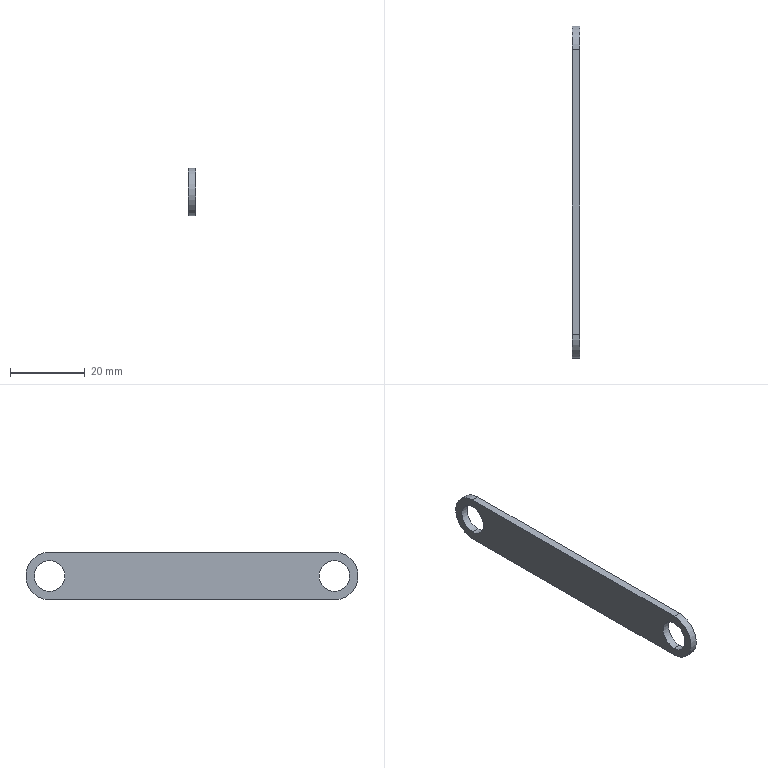Part | SolidWorks | features Extrusion 1 | 1 solid | 10 faces | box 2 x 88.9 x 12.7 mm | volume 1978 mm3 | cylinder 6 | plane 4 | commonest cylinder face diameters 8.2 x4 12.7 x2
STEP:
#1=CARTESIAN_POINT('',(2.,-38.1,4.1));
#2=VERTEX_POINT('',#1);
#3=CARTESIAN_POINT('',(2.,-38.1,-4.1));
#4=VERTEX_POINT('',#3);
#5=CARTESIAN_POINT('',(2.,-38.1,0.));
#6=DIRECTION('',(1.,0.,0.));
#7=DIRECTION('',(0.,0.,-1.));
#8=AXIS2_PLACEMENT_3D('',#5,#6,#7);
#9=CIRCLE('',#8,4.1);
#10=EDGE_CURVE('',#2,#4,#9,.T.);
#11=ORIENTED_EDGE('',*,*,#10,.T.);
#12=CARTESIAN_POINT('',(0.,-38.1,-4.1));
#13=VERTEX_POINT('',#12);
#14=CARTESIAN_POINT('',(2.,-38.1,-4.1));
#15=DIRECTION('',(-1.,0.,0.));
#16=VECTOR('',#15,1000.);
#17=LINE('',#14,#16);
#18=EDGE_CURVE('',#4,#13,#17,.T.);
#19=ORIENTED_EDGE('',*,*,#18,.T.);
#20=CARTESIAN_POINT('',(0.,-38.1,4.1));
#21=VERTEX_POINT('',#20);
#22=CARTESIAN_POINT('',(0.,-38.1,0.));
#23=DIRECTION('',(1.,0.,0.));
#24=DIRECTION('',(0.,0.,-1.));
#25=AXIS2_PLACEMENT_3D('',#22,#23,#24);
#26=CIRCLE('',#25,4.1);
#27=EDGE_CURVE('',#21,#13,#26,.T.);
#28=ORIENTED_EDGE('',*,*,#27,.F.);
#29=CARTESIAN_POINT('',(2.,-38.1,4.1));
#30=DIRECTION('',(-1.,0.,0.));
#31=VECTOR('',#30,1000.);
#32=LINE('',#29,#31);
#33=EDGE_CURVE('',#2,#21,#32,.T.);
#34=ORIENTED_EDGE('',*,*,#33,.F.);
#35=EDGE_LOOP('',(#11,#19,#28,#34));
#36=FACE_OUTER_BOUND('',#35,.T.);
#37=CARTESIAN_POINT('',(2.,-38.1,0.));
#38=DIRECTION('',(-1.,0.,0.));
#39=DIRECTION('',(0.,0.,1.));
#40=AXIS2_PLACEMENT_3D('',#37,#38,#39);
#41=CYLINDRICAL_SURFACE('',#40,4.1);
#42=ADVANCED_FACE('',(#36),#41,.F.);
#43=CARTESIAN_POINT('',(2.,38.1,4.1));
#44=VERTEX_POINT('',#43);
#45=CARTESIAN_POINT('',(2.,38.1,-4.1));
#46=VERTEX_POINT('',#45);
#47=CARTESIAN_POINT('',(2.,38.1,0.));
#48=DIRECTION('',(1.,0.,0.));
#49=DIRECTION('',(0.,0.,-1.));
#50=AXIS2_PLACEMENT_3D('',#47,#48,#49);
#51=CIRCLE('',#50,4.1);
#52=EDGE_CURVE('',#44,#46,#51,.T.);
#53=ORIENTED_EDGE('',*,*,#52,.T.);
#54=CARTESIAN_POINT('',(0.,38.1,-4.1));
#55=VERTEX_POINT('',#54);
#56=CARTESIAN_POINT('',(2.,38.1,-4.1));
#57=DIRECTION('',(-1.,0.,0.));
#58=VECTOR('',#57,1000.);
#59=LINE('',#56,#58);
#60=EDGE_CURVE('',#46,#55,#59,.T.);
#61=ORIENTED_EDGE('',*,*,#60,.T.);
#62=CARTESIAN_POINT('',(0.,38.1,4.1));
#63=VERTEX_POINT('',#62);
#64=CARTESIAN_POINT('',(0.,38.1,0.));
#65=DIRECTION('',(1.,0.,0.));
#66=DIRECTION('',(0.,0.,-1.));
#67=AXIS2_PLACEMENT_3D('',#64,#65,#66);
#68=CIRCLE('',#67,4.1);
#69=EDGE_CURVE('',#63,#55,#68,.T.);
#70=ORIENTED_EDGE('',*,*,#69,.F.);
#71=CARTESIAN_POINT('',(2.,38.1,4.1));
#72=DIRECTION('',(-1.,0.,0.));
#73=VECTOR('',#72,1000.);
#74=LINE('',#71,#73);
#75=EDGE_CURVE('',#44,#63,#74,.T.);
#76=ORIENTED_EDGE('',*,*,#75,.F.);
#77=EDGE_LOOP('',(#53,#61,#70,#76));
#78=FACE_OUTER_BOUND('',#77,.T.);
#79=CARTESIAN_POINT('',(2.,38.1,0.));
#80=DIRECTION('',(-1.,0.,0.));
#81=DIRECTION('',(0.,0.,1.));
#82=AXIS2_PLACEMENT_3D('',#79,#80,#81);
#83=CYLINDRICAL_SURFACE('',#82,4.1);
#84=ADVANCED_FACE('',(#78),#83,.F.);
#85=ORIENTED_EDGE('',*,*,#52,.F.);
#86=CARTESIAN_POINT('',(2.,38.1,0.));
#87=DIRECTION('',(1.,0.,0.));
#88=DIRECTION('',(0.,0.,-1.));
#89=AXIS2_PLACEMENT_3D('',#86,#87,#88);
#90=CIRCLE('',#89,4.1);
#91=EDGE_CURVE('',#46,#44,#90,.T.);
#92=ORIENTED_EDGE('',*,*,#91,.F.);
#93=EDGE_LOOP('',(#85,#92));
#94=FACE_BOUND('',#93,.T.);
#95=CARTESIAN_POINT('',(2.,-38.1,6.35));
#96=VERTEX_POINT('',#95);
#97=CARTESIAN_POINT('',(2.,-38.1,-6.35));
#98=VERTEX_POINT('',#97);
#99=CARTESIAN_POINT('',(2.,-38.1,0.));
#100=DIRECTION('',(1.,0.,0.));
#101=DIRECTION('',(0.,0.,-1.));
#102=AXIS2_PLACEMENT_3D('',#99,#100,#101);
#103=CIRCLE('',#102,6.35);
#104=EDGE_CURVE('',#96,#98,#103,.T.);
#105=ORIENTED_EDGE('',*,*,#104,.T.);
#106=CARTESIAN_POINT('',(2.,38.1,-6.35));
#107=VERTEX_POINT('',#106);
#108=CARTESIAN_POINT('',(2.,-38.1,-6.35));
#109=DIRECTION('',(0.,1.,0.));
#110=VECTOR('',#109,1000.);
#111=LINE('',#108,#110);
#112=EDGE_CURVE('',#98,#107,#111,.T.);
#113=ORIENTED_EDGE('',*,*,#112,.T.);
#114=CARTESIAN_POINT('',(2.,38.1,6.35));
#115=VERTEX_POINT('',#114);
#116=CARTESIAN_POINT('',(2.,38.1,0.));
#117=DIRECTION('',(1.,0.,0.));
#118=DIRECTION('',(0.,0.,-1.));
#119=AXIS2_PLACEMENT_3D('',#116,#117,#118);
#120=CIRCLE('',#119,6.35);
#121=EDGE_CURVE('',#107,#115,#120,.T.);
#122=ORIENTED_EDGE('',*,*,#121,.T.);
#123=CARTESIAN_POINT('',(2.,-38.1,6.35));
#124=DIRECTION('',(0.,-1.,0.));
#125=VECTOR('',#124,1000.);
#126=LINE('',#123,#125);
#127=EDGE_CURVE('',#115,#96,#126,.T.);
#128=ORIENTED_EDGE('',*,*,#127,.T.);
#129=EDGE_LOOP('',(#105,#113,#122,#128));
#130=FACE_OUTER_BOUND('',#129,.T.);
#131=ORIENTED_EDGE('',*,*,#10,.F.);
#132=CARTESIAN_POINT('',(2.,-38.1,0.));
#133=DIRECTION('',(1.,0.,0.));
#134=DIRECTION('',(0.,0.,-1.));
#135=AXIS2_PLACEMENT_3D('',#132,#133,#134);
#136=CIRCLE('',#135,4.1);
#137=EDGE_CURVE('',#4,#2,#136,.T.);
#138=ORIENTED_EDGE('',*,*,#137,.F.);
#139=EDGE_LOOP('',(#131,#138));
#140=FACE_BOUND('',#139,.T.);
#141=CARTESIAN_POINT('',(2.,-38.1,0.));
#142=DIRECTION('',(1.,0.,0.));
#143=DIRECTION('',(0.,0.,-1.));
#144=AXIS2_PLACEMENT_3D('',#141,#142,#143);
#145=PLANE('',#144);
#146=ADVANCED_FACE('',(#94,#130,#140),#145,.T.);
#147=CARTESIAN_POINT('',(0.,-38.1,6.35));
#148=VERTEX_POINT('',#147);
#149=CARTESIAN_POINT('',(0.,-38.1,-6.35));
#150=VERTEX_POINT('',#149);
#151=CARTESIAN_POINT('',(0.,-38.1,0.));
#152=DIRECTION('',(1.,0.,0.));
#153=DIRECTION('',(0.,0.,-1.));
#154=AXIS2_PLACEMENT_3D('',#151,#152,#153);
#155=CIRCLE('',#154,6.35);
#156=EDGE_CURVE('',#148,#150,#155,.T.);
#157=ORIENTED_EDGE('',*,*,#156,.F.);
#158=CARTESIAN_POINT('',(0.,38.1,6.35));
#159=VERTEX_POINT('',#158);
#160=CARTESIAN_POINT('',(0.,-38.1,6.35));
#161=DIRECTION('',(0.,-1.,0.));
#162=VECTOR('',#161,1000.);
#163=LINE('',#160,#162);
#164=EDGE_CURVE('',#159,#148,#163,.T.);
#165=ORIENTED_EDGE('',*,*,#164,.F.);
#166=CARTESIAN_POINT('',(0.,38.1,-6.35));
#167=VERTEX_POINT('',#166);
#168=CARTESIAN_POINT('',(0.,38.1,0.));
#169=DIRECTION('',(1.,0.,0.));
#170=DIRECTION('',(0.,0.,-1.));
#171=AXIS2_PLACEMENT_3D('',#168,#169,#170);
#172=CIRCLE('',#171,6.35);
#173=EDGE_CURVE('',#167,#159,#172,.T.);
#174=ORIENTED_EDGE('',*,*,#173,.F.);
#175=CARTESIAN_POINT('',(0.,-38.1,-6.35));
#176=DIRECTION('',(0.,1.,0.));
#177=VECTOR('',#176,1000.);
#178=LINE('',#175,#177);
#179=EDGE_CURVE('',#150,#167,#178,.T.);
#180=ORIENTED_EDGE('',*,*,#179,.F.);
#181=EDGE_LOOP('',(#157,#165,#174,#180));
#182=FACE_OUTER_BOUND('',#181,.T.);
#183=ORIENTED_EDGE('',*,*,#69,.T.);
#184=CARTESIAN_POINT('',(0.,38.1,0.));
#185=DIRECTION('',(1.,0.,0.));
#186=DIRECTION('',(0.,0.,-1.));
#187=AXIS2_PLACEMENT_3D('',#184,#185,#186);
#188=CIRCLE('',#187,4.1);
#189=EDGE_CURVE('',#55,#63,#188,.T.);
#190=ORIENTED_EDGE('',*,*,#189,.T.);
#191=EDGE_LOOP('',(#183,#190));
#192=FACE_BOUND('',#191,.T.);
#193=ORIENTED_EDGE('',*,*,#27,.T.);
#194=CARTESIAN_POINT('',(0.,-38.1,0.));
#195=DIRECTION('',(1.,0.,0.));
#196=DIRECTION('',(0.,0.,-1.));
#197=AXIS2_PLACEMENT_3D('',#194,#195,#196);
#198=CIRCLE('',#197,4.1);
#199=EDGE_CURVE('',#13,#21,#198,.T.);
#200=ORIENTED_EDGE('',*,*,#199,.T.);
#201=EDGE_LOOP('',(#193,#200));
#202=FACE_BOUND('',#201,.T.);
#203=CARTESIAN_POINT('',(0.,-38.1,0.));
#204=DIRECTION('',(1.,0.,0.));
#205=DIRECTION('',(0.,0.,-1.));
#206=AXIS2_PLACEMENT_3D('',#203,#204,#205);
#207=PLANE('',#206);
#208=ADVANCED_FACE('',(#182,#192,#202),#207,.F.);
#209=ORIENTED_EDGE('',*,*,#156,.T.);
#210=CARTESIAN_POINT('',(2.,-38.1,-6.35));
#211=DIRECTION('',(-1.,0.,0.));
#212=VECTOR('',#211,1000.);
#213=LINE('',#210,#212);
#214=EDGE_CURVE('',#98,#150,#213,.T.);
#215=ORIENTED_EDGE('',*,*,#214,.F.);
#216=ORIENTED_EDGE('',*,*,#104,.F.);
#217=CARTESIAN_POINT('',(2.,-38.1,6.35));
#218=DIRECTION('',(-1.,0.,0.));
#219=VECTOR('',#218,1000.);
#220=LINE('',#217,#219);
#221=EDGE_CURVE('',#96,#148,#220,.T.);
#222=ORIENTED_EDGE('',*,*,#221,.T.);
#223=EDGE_LOOP('',(#209,#215,#216,#222));
#224=FACE_OUTER_BOUND('',#223,.T.);
#225=CARTESIAN_POINT('',(2.,-38.1,0.));
#226=DIRECTION('',(-1.,0.,0.));
#227=DIRECTION('',(0.,0.,1.));
#228=AXIS2_PLACEMENT_3D('',#225,#226,#227);
#229=CYLINDRICAL_SURFACE('',#228,6.35);
#230=ADVANCED_FACE('',(#224),#229,.T.);
#231=ORIENTED_EDGE('',*,*,#179,.T.);
#232=CARTESIAN_POINT('',(2.,38.1,-6.35));
#233=DIRECTION('',(-1.,0.,0.));
#234=VECTOR('',#233,1000.);
#235=LINE('',#232,#234);
#236=EDGE_CURVE('',#107,#167,#235,.T.);
#237=ORIENTED_EDGE('',*,*,#236,.F.);
#238=ORIENTED_EDGE('',*,*,#112,.F.);
#239=ORIENTED_EDGE('',*,*,#214,.T.);
#240=EDGE_LOOP('',(#231,#237,#238,#239));
#241=FACE_OUTER_BOUND('',#240,.T.);
#242=CARTESIAN_POINT('',(2.,-38.1,-6.35));
#243=DIRECTION('',(0.,0.,1.));
#244=DIRECTION('',(0.,-1.,0.));
#245=AXIS2_PLACEMENT_3D('',#242,#243,#244);
#246=PLANE('',#245);
#247=ADVANCED_FACE('',(#241),#246,.F.);
#248=ORIENTED_EDGE('',*,*,#173,.T.);
#249=CARTESIAN_POINT('',(2.,38.1,6.35));
#250=DIRECTION('',(-1.,0.,0.));
#251=VECTOR('',#250,1000.);
#252=LINE('',#249,#251);
#253=EDGE_CURVE('',#115,#159,#252,.T.);
#254=ORIENTED_EDGE('',*,*,#253,.F.);
#255=ORIENTED_EDGE('',*,*,#121,.F.);
#256=ORIENTED_EDGE('',*,*,#236,.T.);
#257=EDGE_LOOP('',(#248,#254,#255,#256));
#258=FACE_OUTER_BOUND('',#257,.T.);
#259=CARTESIAN_POINT('',(2.,38.1,0.));
#260=DIRECTION('',(-1.,0.,0.));
#261=DIRECTION('',(0.,0.,1.));
#262=AXIS2_PLACEMENT_3D('',#259,#260,#261);
#263=CYLINDRICAL_SURFACE('',#262,6.35);
#264=ADVANCED_FACE('',(#258),#263,.T.);
#265=ORIENTED_EDGE('',*,*,#164,.T.);
#266=ORIENTED_EDGE('',*,*,#221,.F.);
#267=ORIENTED_EDGE('',*,*,#127,.F.);
#268=ORIENTED_EDGE('',*,*,#253,.T.);
#269=EDGE_LOOP('',(#265,#266,#267,#268));
#270=FACE_OUTER_BOUND('',#269,.T.);
#271=CARTESIAN_POINT('',(2.,-38.1,6.35));
#272=DIRECTION('',(0.,0.,-1.));
#273=DIRECTION('',(0.,1.,0.));
#274=AXIS2_PLACEMENT_3D('',#271,#272,#273);
#275=PLANE('',#274);
#276=ADVANCED_FACE('',(#270),#275,.F.);
#277=ORIENTED_EDGE('',*,*,#60,.F.);
#278=ORIENTED_EDGE('',*,*,#91,.T.);
#279=ORIENTED_EDGE('',*,*,#75,.T.);
#280=ORIENTED_EDGE('',*,*,#189,.F.);
#281=EDGE_LOOP('',(#277,#278,#279,#280));
#282=FACE_OUTER_BOUND('',#281,.T.);
#283=CARTESIAN_POINT('',(2.,38.1,0.));
#284=DIRECTION('',(-1.,0.,0.));
#285=DIRECTION('',(0.,0.,1.));
#286=AXIS2_PLACEMENT_3D('',#283,#284,#285);
#287=CYLINDRICAL_SURFACE('',#286,4.1);
#288=ADVANCED_FACE('',(#282),#287,.F.);
#289=ORIENTED_EDGE('',*,*,#18,.F.);
#290=ORIENTED_EDGE('',*,*,#137,.T.);
#291=ORIENTED_EDGE('',*,*,#33,.T.);
#292=ORIENTED_EDGE('',*,*,#199,.F.);
#293=EDGE_LOOP('',(#289,#290,#291,#292));
#294=FACE_OUTER_BOUND('',#293,.T.);
#295=CARTESIAN_POINT('',(2.,-38.1,0.));
#296=DIRECTION('',(-1.,0.,0.));
#297=DIRECTION('',(0.,0.,1.));
#298=AXIS2_PLACEMENT_3D('',#295,#296,#297);
#299=CYLINDRICAL_SURFACE('',#298,4.1);
#300=ADVANCED_FACE('',(#294),#299,.F.);
#301=CLOSED_SHELL('',(#42,#84,#146,#208,#230,#247,#264,#276,#288,#300));
#302=MANIFOLD_SOLID_BREP('',#301);
#303=CARTESIAN_POINT('',(0.,0.,0.));
#304=DIRECTION('',(0.,0.,1.));
#305=DIRECTION('',(1.,0.,0.));
#306=AXIS2_PLACEMENT_3D('',#303,#304,#305);
#307=(LENGTH_UNIT()NAMED_UNIT(*)SI_UNIT(.MILLI.,.METRE.));
#308=UNCERTAINTY_MEASURE_WITH_UNIT(LENGTH_MEASURE(0.00001),#307,'','');
#309=(NAMED_UNIT(*)PLANE_ANGLE_UNIT()SI_UNIT($,.RADIAN.));
#310=(NAMED_UNIT(*)SI_UNIT($,.STERADIAN.)SOLID_ANGLE_UNIT());
#311=(GEOMETRIC_REPRESENTATION_CONTEXT(3)GLOBAL_UNCERTAINTY_ASSIGNED_CONTEXT((#308))GLOBAL_UNIT_ASSIGNED_CONTEXT((#307,#309,#310))REPRESENTATION_CONTEXT('',''));
#312=ADVANCED_BREP_SHAPE_REPRESENTATION('',(#302,#306),#311);